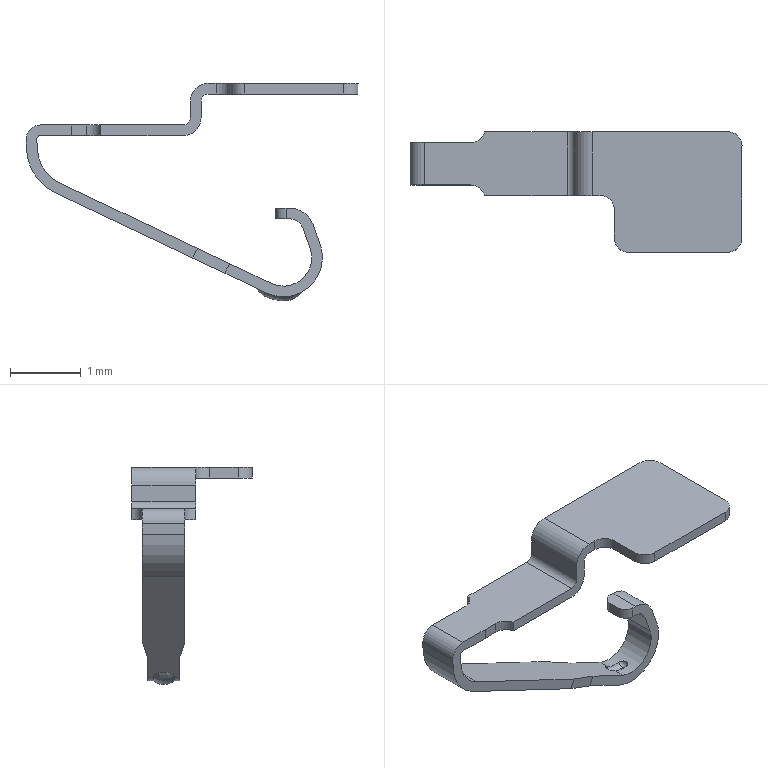Part | STEP file | p9-frame-01 | 1 solid | 62 faces | box 4.684 x 1.7 x 3.066 mm | volume 1.347 mm3 | plane 28 | cylinder 26 | spline 8 | commonest cylinder face diameters 0.4 x9 1.1 x3 0.157 x2 0.2 x2 0.3 x2 0.457 x2